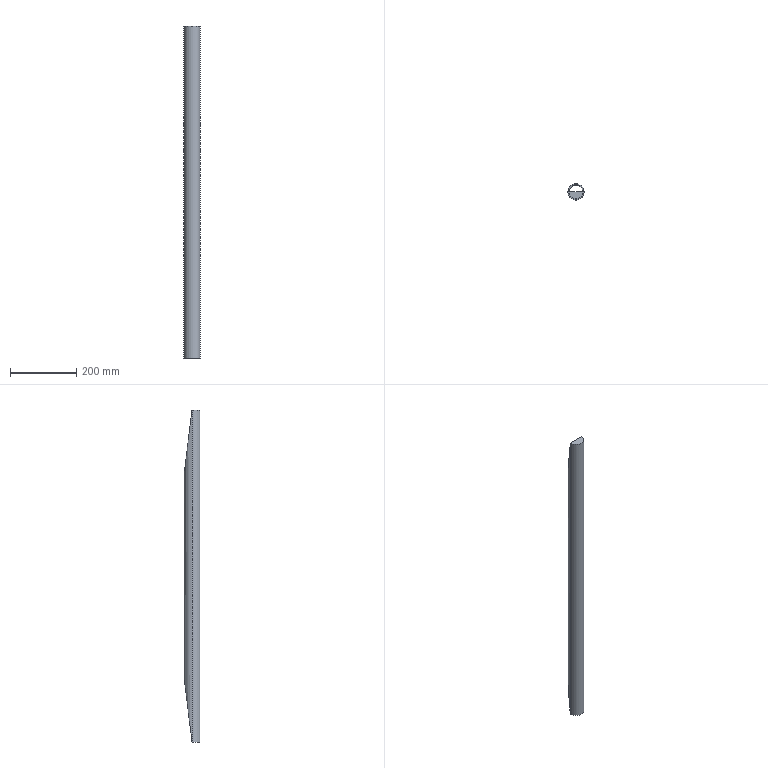Part | SolidWorks | features Extrusion 1, ICE 1, Shell 1 | 1 solid | 10 faces | box 48.3 x 48.3 x 1000 mm | volume 380976 mm3 | plane 6 | cylinder 4 | commonest cylinder face diameters 42.3 x2 48.3 x2
STEP:
#1=CARTESIAN_POINT('',(-21.15,0.,997.));
#2=VERTEX_POINT('',#1);
#3=CARTESIAN_POINT('',(21.15,0.,997.));
#4=VERTEX_POINT('',#3);
#5=CARTESIAN_POINT('',(0.,0.,997.));
#6=DIRECTION('',(0.,0.,1.));
#7=DIRECTION('',(1.,0.,0.));
#8=AXIS2_PLACEMENT_3D('',#5,#6,#7);
#9=CIRCLE('',#8,21.15);
#10=EDGE_CURVE('',#2,#4,#9,.T.);
#11=ORIENTED_EDGE('',*,*,#10,.T.);
#12=CARTESIAN_POINT('',(21.15,0.,3.));
#13=VERTEX_POINT('',#12);
#14=CARTESIAN_POINT('',(21.15,0.,1000.));
#15=DIRECTION('',(0.,0.,-1.));
#16=VECTOR('',#15,1000.);
#17=LINE('',#14,#16);
#18=EDGE_CURVE('',#4,#13,#17,.T.);
#19=ORIENTED_EDGE('',*,*,#18,.T.);
#20=CARTESIAN_POINT('',(-21.15,0.,3.));
#21=VERTEX_POINT('',#20);
#22=CARTESIAN_POINT('',(0.,0.,3.));
#23=DIRECTION('',(0.,0.,1.));
#24=DIRECTION('',(1.,0.,0.));
#25=AXIS2_PLACEMENT_3D('',#22,#23,#24);
#26=CIRCLE('',#25,21.15);
#27=EDGE_CURVE('',#21,#13,#26,.T.);
#28=ORIENTED_EDGE('',*,*,#27,.F.);
#29=CARTESIAN_POINT('',(-21.15,0.,1000.));
#30=DIRECTION('',(0.,0.,-1.));
#31=VECTOR('',#30,1000.);
#32=LINE('',#29,#31);
#33=EDGE_CURVE('',#2,#21,#32,.T.);
#34=ORIENTED_EDGE('',*,*,#33,.F.);
#35=EDGE_LOOP('',(#11,#19,#28,#34));
#36=FACE_OUTER_BOUND('',#35,.T.);
#37=CARTESIAN_POINT('',(0.,0.,1000.));
#38=DIRECTION('',(0.,0.,-1.));
#39=DIRECTION('',(-1.,0.,0.));
#40=AXIS2_PLACEMENT_3D('',#37,#38,#39);
#41=CYLINDRICAL_SURFACE('',#40,21.15);
#42=ADVANCED_FACE('',(#36),#41,.F.);
#43=CARTESIAN_POINT('',(-24.15,0.,1000.));
#44=VERTEX_POINT('',#43);
#45=CARTESIAN_POINT('',(24.15,0.,1000.));
#46=VERTEX_POINT('',#45);
#47=CARTESIAN_POINT('',(-24.15,0.,1000.));
#48=CARTESIAN_POINT('',(-24.15,48.3,606.628));
#49=CARTESIAN_POINT('',(24.15,48.3,606.628));
#50=CARTESIAN_POINT('',(24.15,0.,1000.));
#51=(BOUNDED_CURVE()B_SPLINE_CURVE(3,(#47,#48,#49,#50),.UNSPECIFIED.,.F.,.T.)B_SPLINE_CURVE_WITH_KNOTS((4,4),(4.712,7.854),.UNSPECIFIED.)CURVE()GEOMETRIC_REPRESENTATION_ITEM()RATIONAL_B_SPLINE_CURVE((1.,0.3333,0.3333,1.))REPRESENTATION_ITEM(''));
#52=EDGE_CURVE('',#44,#46,#51,.T.);
#53=ORIENTED_EDGE('',*,*,#52,.T.);
#54=CARTESIAN_POINT('',(24.15,0.,0.));
#55=VERTEX_POINT('',#54);
#56=CARTESIAN_POINT('',(24.15,0.,1000.));
#57=DIRECTION('',(0.,0.,-1.));
#58=VECTOR('',#57,1000.);
#59=LINE('',#56,#58);
#60=EDGE_CURVE('',#46,#55,#59,.T.);
#61=ORIENTED_EDGE('',*,*,#60,.T.);
#62=CARTESIAN_POINT('',(-24.15,0.,0.));
#63=VERTEX_POINT('',#62);
#64=CARTESIAN_POINT('',(24.15,0.,0.));
#65=CARTESIAN_POINT('',(24.15,48.3,393.372));
#66=CARTESIAN_POINT('',(-24.15,48.3,393.372));
#67=CARTESIAN_POINT('',(-24.15,0.,0.));
#68=(BOUNDED_CURVE()B_SPLINE_CURVE(3,(#64,#65,#66,#67),.UNSPECIFIED.,.F.,.T.)B_SPLINE_CURVE_WITH_KNOTS((4,4),(1.571,4.712),.UNSPECIFIED.)CURVE()GEOMETRIC_REPRESENTATION_ITEM()RATIONAL_B_SPLINE_CURVE((1.,0.3333,0.3333,1.))REPRESENTATION_ITEM(''));
#69=EDGE_CURVE('',#55,#63,#68,.T.);
#70=ORIENTED_EDGE('',*,*,#69,.T.);
#71=CARTESIAN_POINT('',(-24.15,0.,1000.));
#72=DIRECTION('',(0.,0.,-1.));
#73=VECTOR('',#72,1000.);
#74=LINE('',#71,#73);
#75=EDGE_CURVE('',#44,#63,#74,.T.);
#76=ORIENTED_EDGE('',*,*,#75,.F.);
#77=EDGE_LOOP('',(#53,#61,#70,#76));
#78=FACE_OUTER_BOUND('',#77,.T.);
#79=CARTESIAN_POINT('',(0.,0.,1000.));
#80=DIRECTION('',(0.,0.,-1.));
#81=DIRECTION('',(-1.,0.,0.));
#82=AXIS2_PLACEMENT_3D('',#79,#80,#81);
#83=CYLINDRICAL_SURFACE('',#82,24.15);
#84=ADVANCED_FACE('',(#78),#83,.T.);
#85=ORIENTED_EDGE('',*,*,#60,.F.);
#86=CARTESIAN_POINT('',(0.,0.,1000.));
#87=DIRECTION('',(0.,0.,1.));
#88=DIRECTION('',(1.,0.,0.));
#89=AXIS2_PLACEMENT_3D('',#86,#87,#88);
#90=CIRCLE('',#89,24.15);
#91=EDGE_CURVE('',#44,#46,#90,.T.);
#92=ORIENTED_EDGE('',*,*,#91,.F.);
#93=ORIENTED_EDGE('',*,*,#75,.T.);
#94=CARTESIAN_POINT('',(0.,0.,0.));
#95=DIRECTION('',(0.,0.,1.));
#96=DIRECTION('',(1.,0.,0.));
#97=AXIS2_PLACEMENT_3D('',#94,#95,#96);
#98=CIRCLE('',#97,24.15);
#99=EDGE_CURVE('',#63,#55,#98,.T.);
#100=ORIENTED_EDGE('',*,*,#99,.T.);
#101=EDGE_LOOP('',(#85,#92,#93,#100));
#102=FACE_OUTER_BOUND('',#101,.T.);
#103=CARTESIAN_POINT('',(0.,0.,1000.));
#104=DIRECTION('',(0.,0.,-1.));
#105=DIRECTION('',(-1.,0.,0.));
#106=AXIS2_PLACEMENT_3D('',#103,#104,#105);
#107=CYLINDRICAL_SURFACE('',#106,24.15);
#108=ADVANCED_FACE('',(#102),#107,.T.);
#109=CARTESIAN_POINT('',(0.,0.,1000.));
#110=DIRECTION('',(1.,0.,0.));
#111=VECTOR('',#110,1000.);
#112=LINE('',#109,#111);
#113=EDGE_CURVE('',#44,#46,#112,.T.);
#114=ORIENTED_EDGE('',*,*,#113,.F.);
#115=ORIENTED_EDGE('',*,*,#91,.T.);
#116=EDGE_LOOP('',(#114,#115));
#117=FACE_OUTER_BOUND('',#116,.T.);
#118=CARTESIAN_POINT('',(0.,0.,1000.));
#119=DIRECTION('',(0.,0.,1.));
#120=DIRECTION('',(1.,0.,0.));
#121=AXIS2_PLACEMENT_3D('',#118,#119,#120);
#122=PLANE('',#121);
#123=ADVANCED_FACE('',(#117),#122,.T.);
#124=ORIENTED_EDGE('',*,*,#99,.F.);
#125=CARTESIAN_POINT('',(0.,0.,0.));
#126=DIRECTION('',(1.,0.,0.));
#127=VECTOR('',#126,1000.);
#128=LINE('',#125,#127);
#129=EDGE_CURVE('',#63,#55,#128,.T.);
#130=ORIENTED_EDGE('',*,*,#129,.T.);
#131=EDGE_LOOP('',(#124,#130));
#132=FACE_OUTER_BOUND('',#131,.T.);
#133=CARTESIAN_POINT('',(0.,0.,0.));
#134=DIRECTION('',(0.,0.,1.));
#135=DIRECTION('',(1.,0.,0.));
#136=AXIS2_PLACEMENT_3D('',#133,#134,#135);
#137=PLANE('',#136);
#138=ADVANCED_FACE('',(#132),#137,.F.);
#139=CARTESIAN_POINT('',(21.147,0.3684,3.));
#140=VERTEX_POINT('',#139);
#141=CARTESIAN_POINT('',(-21.147,0.3684,3.));
#142=VERTEX_POINT('',#141);
#143=CARTESIAN_POINT('',(21.147,0.3684,3.));
#144=CARTESIAN_POINT('',(20.435,41.232,335.809));
#145=CARTESIAN_POINT('',(-20.435,41.232,335.809));
#146=CARTESIAN_POINT('',(-21.147,0.3684,3.));
#147=(BOUNDED_CURVE()B_SPLINE_CURVE(3,(#143,#144,#145,#146),.UNSPECIFIED.,.F.,.T.)B_SPLINE_CURVE_WITH_KNOTS((4,4),(1.588,4.695),.UNSPECIFIED.)CURVE()GEOMETRIC_REPRESENTATION_ITEM()RATIONAL_B_SPLINE_CURVE((1.,0.3449,0.3449,1.))REPRESENTATION_ITEM(''));
#148=EDGE_CURVE('',#140,#142,#147,.T.);
#149=ORIENTED_EDGE('',*,*,#148,.T.);
#150=CARTESIAN_POINT('',(0.,0.3684,3.));
#151=DIRECTION('',(1.,0.,0.));
#152=VECTOR('',#151,1000.);
#153=LINE('',#150,#152);
#154=EDGE_CURVE('',#142,#140,#153,.T.);
#155=ORIENTED_EDGE('',*,*,#154,.T.);
#156=EDGE_LOOP('',(#149,#155));
#157=FACE_BOUND('',#156,.T.);
#158=ORIENTED_EDGE('',*,*,#129,.F.);
#159=ORIENTED_EDGE('',*,*,#69,.F.);
#160=EDGE_LOOP('',(#158,#159));
#161=FACE_OUTER_BOUND('',#160,.T.);
#162=CARTESIAN_POINT('',(-500.,0.,0.));
#163=DIRECTION('',(0.,-0.9925,0.1219));
#164=DIRECTION('',(0.,-0.1219,-0.9925));
#165=AXIS2_PLACEMENT_3D('',#162,#163,#164);
#166=PLANE('',#165);
#167=ADVANCED_FACE('',(#157,#161),#166,.F.);
#168=CARTESIAN_POINT('',(-21.147,0.3684,997.));
#169=VERTEX_POINT('',#168);
#170=CARTESIAN_POINT('',(21.147,0.3684,997.));
#171=VERTEX_POINT('',#170);
#172=CARTESIAN_POINT('',(0.,0.3684,997.));
#173=DIRECTION('',(1.,0.,0.));
#174=VECTOR('',#173,1000.);
#175=LINE('',#172,#174);
#176=EDGE_CURVE('',#169,#171,#175,.T.);
#177=ORIENTED_EDGE('',*,*,#176,.F.);
#178=CARTESIAN_POINT('',(-21.147,0.3684,997.));
#179=CARTESIAN_POINT('',(-20.435,41.232,664.191));
#180=CARTESIAN_POINT('',(20.435,41.232,664.191));
#181=CARTESIAN_POINT('',(21.147,0.3684,997.));
#182=(BOUNDED_CURVE()B_SPLINE_CURVE(3,(#178,#179,#180,#181),.UNSPECIFIED.,.F.,.T.)B_SPLINE_CURVE_WITH_KNOTS((4,4),(4.73,7.837),.UNSPECIFIED.)CURVE()GEOMETRIC_REPRESENTATION_ITEM()RATIONAL_B_SPLINE_CURVE((1.,0.3449,0.3449,1.))REPRESENTATION_ITEM(''));
#183=EDGE_CURVE('',#169,#171,#182,.T.);
#184=ORIENTED_EDGE('',*,*,#183,.T.);
#185=EDGE_LOOP('',(#177,#184));
#186=FACE_BOUND('',#185,.T.);
#187=ORIENTED_EDGE('',*,*,#52,.F.);
#188=ORIENTED_EDGE('',*,*,#113,.T.);
#189=EDGE_LOOP('',(#187,#188));
#190=FACE_OUTER_BOUND('',#189,.T.);
#191=CARTESIAN_POINT('',(-500.,0.,1000.));
#192=DIRECTION('',(0.,-0.9925,-0.1219));
#193=DIRECTION('',(0.,0.1219,-0.9925));
#194=AXIS2_PLACEMENT_3D('',#191,#192,#193);
#195=PLANE('',#194);
#196=ADVANCED_FACE('',(#186,#190),#195,.F.);
#197=ORIENTED_EDGE('',*,*,#18,.F.);
#198=CARTESIAN_POINT('',(0.,0.,997.));
#199=DIRECTION('',(0.,0.,1.));
#200=DIRECTION('',(1.,0.,0.));
#201=AXIS2_PLACEMENT_3D('',#198,#199,#200);
#202=CIRCLE('',#201,21.15);
#203=EDGE_CURVE('',#4,#171,#202,.T.);
#204=ORIENTED_EDGE('',*,*,#203,.T.);
#205=ORIENTED_EDGE('',*,*,#183,.F.);
#206=CARTESIAN_POINT('',(0.,0.,997.));
#207=DIRECTION('',(0.,0.,1.));
#208=DIRECTION('',(1.,0.,0.));
#209=AXIS2_PLACEMENT_3D('',#206,#207,#208);
#210=CIRCLE('',#209,21.15);
#211=EDGE_CURVE('',#169,#2,#210,.T.);
#212=ORIENTED_EDGE('',*,*,#211,.T.);
#213=ORIENTED_EDGE('',*,*,#33,.T.);
#214=CARTESIAN_POINT('',(0.,0.,3.));
#215=DIRECTION('',(0.,0.,1.));
#216=DIRECTION('',(1.,0.,0.));
#217=AXIS2_PLACEMENT_3D('',#214,#215,#216);
#218=CIRCLE('',#217,21.15);
#219=EDGE_CURVE('',#142,#21,#218,.T.);
#220=ORIENTED_EDGE('',*,*,#219,.F.);
#221=ORIENTED_EDGE('',*,*,#148,.F.);
#222=CARTESIAN_POINT('',(0.,0.,3.));
#223=DIRECTION('',(0.,0.,1.));
#224=DIRECTION('',(1.,0.,0.));
#225=AXIS2_PLACEMENT_3D('',#222,#223,#224);
#226=CIRCLE('',#225,21.15);
#227=EDGE_CURVE('',#13,#140,#226,.T.);
#228=ORIENTED_EDGE('',*,*,#227,.F.);
#229=EDGE_LOOP('',(#197,#204,#205,#212,#213,#220,#221,#228));
#230=FACE_OUTER_BOUND('',#229,.T.);
#231=CARTESIAN_POINT('',(0.,0.,1000.));
#232=DIRECTION('',(0.,0.,-1.));
#233=DIRECTION('',(-1.,0.,0.));
#234=AXIS2_PLACEMENT_3D('',#231,#232,#233);
#235=CYLINDRICAL_SURFACE('',#234,21.15);
#236=ADVANCED_FACE('',(#230),#235,.F.);
#237=ORIENTED_EDGE('',*,*,#176,.T.);
#238=ORIENTED_EDGE('',*,*,#203,.F.);
#239=ORIENTED_EDGE('',*,*,#10,.F.);
#240=ORIENTED_EDGE('',*,*,#211,.F.);
#241=EDGE_LOOP('',(#237,#238,#239,#240));
#242=FACE_OUTER_BOUND('',#241,.T.);
#243=CARTESIAN_POINT('',(0.,0.,997.));
#244=DIRECTION('',(0.,0.,1.));
#245=DIRECTION('',(1.,0.,0.));
#246=AXIS2_PLACEMENT_3D('',#243,#244,#245);
#247=PLANE('',#246);
#248=ADVANCED_FACE('',(#242),#247,.F.);
#249=ORIENTED_EDGE('',*,*,#219,.T.);
#250=ORIENTED_EDGE('',*,*,#27,.T.);
#251=ORIENTED_EDGE('',*,*,#227,.T.);
#252=ORIENTED_EDGE('',*,*,#154,.F.);
#253=EDGE_LOOP('',(#249,#250,#251,#252));
#254=FACE_OUTER_BOUND('',#253,.T.);
#255=CARTESIAN_POINT('',(0.,0.,3.));
#256=DIRECTION('',(0.,0.,1.));
#257=DIRECTION('',(1.,0.,0.));
#258=AXIS2_PLACEMENT_3D('',#255,#256,#257);
#259=PLANE('',#258);
#260=ADVANCED_FACE('',(#254),#259,.T.);
#261=CLOSED_SHELL('',(#42,#84,#108,#123,#138,#167,#196,#236,#248,#260));
#262=MANIFOLD_SOLID_BREP('',#261);
#263=CARTESIAN_POINT('',(0.,0.,0.));
#264=DIRECTION('',(0.,0.,1.));
#265=DIRECTION('',(1.,0.,0.));
#266=AXIS2_PLACEMENT_3D('',#263,#264,#265);
#267=(LENGTH_UNIT()NAMED_UNIT(*)SI_UNIT(.MILLI.,.METRE.));
#268=UNCERTAINTY_MEASURE_WITH_UNIT(LENGTH_MEASURE(0.00001),#267,'','');
#269=(NAMED_UNIT(*)PLANE_ANGLE_UNIT()SI_UNIT($,.RADIAN.));
#270=(NAMED_UNIT(*)SI_UNIT($,.STERADIAN.)SOLID_ANGLE_UNIT());
#271=(GEOMETRIC_REPRESENTATION_CONTEXT(3)GLOBAL_UNCERTAINTY_ASSIGNED_CONTEXT((#268))GLOBAL_UNIT_ASSIGNED_CONTEXT((#267,#269,#270))REPRESENTATION_CONTEXT('',''));
#272=ADVANCED_BREP_SHAPE_REPRESENTATION('',(#262,#266),#271);